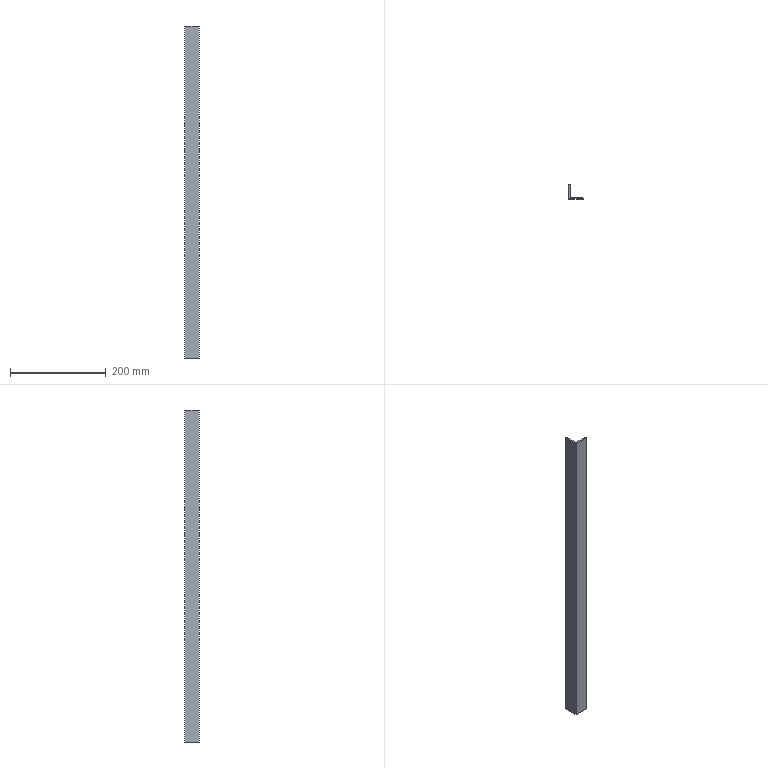Part | SolidWorks | features Extrusion 1 | 1 solid | 11 faces | box 30 x 30 x 692 mm | volume 117738 mm3 | plane 8 | cylinder 3 | commonest cylinder face diameters 4 x3
STEP:
#1=CARTESIAN_POINT('',(0.,30.,0.));
#2=VERTEX_POINT('',#1);
#3=CARTESIAN_POINT('',(0.,0.,0.));
#4=VERTEX_POINT('',#3);
#5=CARTESIAN_POINT('',(0.,0.,0.));
#6=DIRECTION('',(0.,-1.,0.));
#7=VECTOR('',#6,1000.);
#8=LINE('',#5,#7);
#9=EDGE_CURVE('',#2,#4,#8,.T.);
#10=ORIENTED_EDGE('',*,*,#9,.T.);
#11=CARTESIAN_POINT('',(0.,0.,692.));
#12=VERTEX_POINT('',#11);
#13=CARTESIAN_POINT('',(0.,0.,692.));
#14=DIRECTION('',(0.,0.,-1.));
#15=VECTOR('',#14,1000.);
#16=LINE('',#13,#15);
#17=EDGE_CURVE('',#12,#4,#16,.T.);
#18=ORIENTED_EDGE('',*,*,#17,.F.);
#19=CARTESIAN_POINT('',(0.,30.,692.));
#20=VERTEX_POINT('',#19);
#21=CARTESIAN_POINT('',(0.,0.,692.));
#22=DIRECTION('',(0.,-1.,0.));
#23=VECTOR('',#22,1000.);
#24=LINE('',#21,#23);
#25=EDGE_CURVE('',#20,#12,#24,.T.);
#26=ORIENTED_EDGE('',*,*,#25,.F.);
#27=CARTESIAN_POINT('',(0.,30.,692.));
#28=DIRECTION('',(0.,0.,-1.));
#29=VECTOR('',#28,1000.);
#30=LINE('',#27,#29);
#31=EDGE_CURVE('',#20,#2,#30,.T.);
#32=ORIENTED_EDGE('',*,*,#31,.T.);
#33=EDGE_LOOP('',(#10,#18,#26,#32));
#34=FACE_OUTER_BOUND('',#33,.T.);
#35=CARTESIAN_POINT('',(0.,0.,692.));
#36=DIRECTION('',(1.,0.,0.));
#37=DIRECTION('',(0.,0.,-1.));
#38=AXIS2_PLACEMENT_3D('',#35,#36,#37);
#39=PLANE('',#38);
#40=ADVANCED_FACE('',(#34),#39,.F.);
#41=CARTESIAN_POINT('',(30.,0.,0.));
#42=VERTEX_POINT('',#41);
#43=CARTESIAN_POINT('',(0.,0.,0.));
#44=DIRECTION('',(1.,0.,0.));
#45=VECTOR('',#44,1000.);
#46=LINE('',#43,#45);
#47=EDGE_CURVE('',#4,#42,#46,.T.);
#48=ORIENTED_EDGE('',*,*,#47,.T.);
#49=CARTESIAN_POINT('',(30.,0.,692.));
#50=VERTEX_POINT('',#49);
#51=CARTESIAN_POINT('',(30.,0.,692.));
#52=DIRECTION('',(0.,0.,-1.));
#53=VECTOR('',#52,1000.);
#54=LINE('',#51,#53);
#55=EDGE_CURVE('',#50,#42,#54,.T.);
#56=ORIENTED_EDGE('',*,*,#55,.F.);
#57=CARTESIAN_POINT('',(0.,0.,692.));
#58=DIRECTION('',(1.,0.,0.));
#59=VECTOR('',#58,1000.);
#60=LINE('',#57,#59);
#61=EDGE_CURVE('',#12,#50,#60,.T.);
#62=ORIENTED_EDGE('',*,*,#61,.F.);
#63=ORIENTED_EDGE('',*,*,#17,.T.);
#64=EDGE_LOOP('',(#48,#56,#62,#63));
#65=FACE_OUTER_BOUND('',#64,.T.);
#66=CARTESIAN_POINT('',(0.,0.,692.));
#67=DIRECTION('',(0.,1.,0.));
#68=DIRECTION('',(0.,0.,1.));
#69=AXIS2_PLACEMENT_3D('',#66,#67,#68);
#70=PLANE('',#69);
#71=ADVANCED_FACE('',(#65),#70,.F.);
#72=CARTESIAN_POINT('',(30.,1.,0.));
#73=VERTEX_POINT('',#72);
#74=CARTESIAN_POINT('',(30.,1.,0.));
#75=DIRECTION('',(0.,1.,0.));
#76=VECTOR('',#75,1000.);
#77=LINE('',#74,#76);
#78=EDGE_CURVE('',#42,#73,#77,.T.);
#79=ORIENTED_EDGE('',*,*,#78,.T.);
#80=CARTESIAN_POINT('',(30.,1.,692.));
#81=VERTEX_POINT('',#80);
#82=CARTESIAN_POINT('',(30.,1.,692.));
#83=DIRECTION('',(0.,0.,-1.));
#84=VECTOR('',#83,1000.);
#85=LINE('',#82,#84);
#86=EDGE_CURVE('',#81,#73,#85,.T.);
#87=ORIENTED_EDGE('',*,*,#86,.F.);
#88=CARTESIAN_POINT('',(30.,1.,692.));
#89=DIRECTION('',(0.,1.,0.));
#90=VECTOR('',#89,1000.);
#91=LINE('',#88,#90);
#92=EDGE_CURVE('',#50,#81,#91,.T.);
#93=ORIENTED_EDGE('',*,*,#92,.F.);
#94=ORIENTED_EDGE('',*,*,#55,.T.);
#95=EDGE_LOOP('',(#79,#87,#93,#94));
#96=FACE_OUTER_BOUND('',#95,.T.);
#97=CARTESIAN_POINT('',(30.,1.,692.));
#98=DIRECTION('',(-1.,0.,0.));
#99=DIRECTION('',(0.,0.,1.));
#100=AXIS2_PLACEMENT_3D('',#97,#98,#99);
#101=PLANE('',#100);
#102=ADVANCED_FACE('',(#96),#101,.F.);
#103=CARTESIAN_POINT('',(28.,3.,0.));
#104=VERTEX_POINT('',#103);
#105=CARTESIAN_POINT('',(28.,1.,0.));
#106=DIRECTION('',(0.,0.,1.));
#107=DIRECTION('',(1.,0.,0.));
#108=AXIS2_PLACEMENT_3D('',#105,#106,#107);
#109=CIRCLE('',#108,2.);
#110=EDGE_CURVE('',#73,#104,#109,.T.);
#111=ORIENTED_EDGE('',*,*,#110,.T.);
#112=CARTESIAN_POINT('',(28.,3.,692.));
#113=VERTEX_POINT('',#112);
#114=CARTESIAN_POINT('',(28.,3.,692.));
#115=DIRECTION('',(0.,0.,-1.));
#116=VECTOR('',#115,1000.);
#117=LINE('',#114,#116);
#118=EDGE_CURVE('',#113,#104,#117,.T.);
#119=ORIENTED_EDGE('',*,*,#118,.F.);
#120=CARTESIAN_POINT('',(28.,1.,692.));
#121=DIRECTION('',(0.,0.,1.));
#122=DIRECTION('',(1.,0.,0.));
#123=AXIS2_PLACEMENT_3D('',#120,#121,#122);
#124=CIRCLE('',#123,2.);
#125=EDGE_CURVE('',#81,#113,#124,.T.);
#126=ORIENTED_EDGE('',*,*,#125,.F.);
#127=ORIENTED_EDGE('',*,*,#86,.T.);
#128=EDGE_LOOP('',(#111,#119,#126,#127));
#129=FACE_OUTER_BOUND('',#128,.T.);
#130=CARTESIAN_POINT('',(28.,1.,692.));
#131=DIRECTION('',(0.,0.,-1.));
#132=DIRECTION('',(-1.,0.,0.));
#133=AXIS2_PLACEMENT_3D('',#130,#131,#132);
#134=CYLINDRICAL_SURFACE('',#133,2.);
#135=ADVANCED_FACE('',(#129),#134,.T.);
#136=CARTESIAN_POINT('',(5.,3.,0.));
#137=VERTEX_POINT('',#136);
#138=CARTESIAN_POINT('',(5.,3.,0.));
#139=DIRECTION('',(-1.,0.,0.));
#140=VECTOR('',#139,1000.);
#141=LINE('',#138,#140);
#142=EDGE_CURVE('',#104,#137,#141,.T.);
#143=ORIENTED_EDGE('',*,*,#142,.T.);
#144=CARTESIAN_POINT('',(5.,3.,692.));
#145=VERTEX_POINT('',#144);
#146=CARTESIAN_POINT('',(5.,3.,692.));
#147=DIRECTION('',(0.,0.,-1.));
#148=VECTOR('',#147,1000.);
#149=LINE('',#146,#148);
#150=EDGE_CURVE('',#145,#137,#149,.T.);
#151=ORIENTED_EDGE('',*,*,#150,.F.);
#152=CARTESIAN_POINT('',(5.,3.,692.));
#153=DIRECTION('',(-1.,0.,0.));
#154=VECTOR('',#153,1000.);
#155=LINE('',#152,#154);
#156=EDGE_CURVE('',#113,#145,#155,.T.);
#157=ORIENTED_EDGE('',*,*,#156,.F.);
#158=ORIENTED_EDGE('',*,*,#118,.T.);
#159=EDGE_LOOP('',(#143,#151,#157,#158));
#160=FACE_OUTER_BOUND('',#159,.T.);
#161=CARTESIAN_POINT('',(5.,3.,692.));
#162=DIRECTION('',(0.,-1.,0.));
#163=DIRECTION('',(0.,0.,-1.));
#164=AXIS2_PLACEMENT_3D('',#161,#162,#163);
#165=PLANE('',#164);
#166=ADVANCED_FACE('',(#160),#165,.F.);
#167=CARTESIAN_POINT('',(3.,5.,0.));
#168=VERTEX_POINT('',#167);
#169=CARTESIAN_POINT('',(5.,5.,0.));
#170=DIRECTION('',(0.,0.,-1.));
#171=DIRECTION('',(-1.,0.,0.));
#172=AXIS2_PLACEMENT_3D('',#169,#170,#171);
#173=CIRCLE('',#172,2.);
#174=EDGE_CURVE('',#137,#168,#173,.T.);
#175=ORIENTED_EDGE('',*,*,#174,.T.);
#176=CARTESIAN_POINT('',(3.,5.,692.));
#177=VERTEX_POINT('',#176);
#178=CARTESIAN_POINT('',(3.,5.,692.));
#179=DIRECTION('',(0.,0.,-1.));
#180=VECTOR('',#179,1000.);
#181=LINE('',#178,#180);
#182=EDGE_CURVE('',#177,#168,#181,.T.);
#183=ORIENTED_EDGE('',*,*,#182,.F.);
#184=CARTESIAN_POINT('',(5.,5.,692.));
#185=DIRECTION('',(0.,0.,-1.));
#186=DIRECTION('',(-1.,0.,0.));
#187=AXIS2_PLACEMENT_3D('',#184,#185,#186);
#188=CIRCLE('',#187,2.);
#189=EDGE_CURVE('',#145,#177,#188,.T.);
#190=ORIENTED_EDGE('',*,*,#189,.F.);
#191=ORIENTED_EDGE('',*,*,#150,.T.);
#192=EDGE_LOOP('',(#175,#183,#190,#191));
#193=FACE_OUTER_BOUND('',#192,.T.);
#194=CARTESIAN_POINT('',(5.,5.,692.));
#195=DIRECTION('',(0.,0.,-1.));
#196=DIRECTION('',(-1.,0.,0.));
#197=AXIS2_PLACEMENT_3D('',#194,#195,#196);
#198=CYLINDRICAL_SURFACE('',#197,2.);
#199=ADVANCED_FACE('',(#193),#198,.F.);
#200=CARTESIAN_POINT('',(3.,28.,0.));
#201=VERTEX_POINT('',#200);
#202=CARTESIAN_POINT('',(3.,5.,0.));
#203=DIRECTION('',(0.,1.,0.));
#204=VECTOR('',#203,1000.);
#205=LINE('',#202,#204);
#206=EDGE_CURVE('',#168,#201,#205,.T.);
#207=ORIENTED_EDGE('',*,*,#206,.T.);
#208=CARTESIAN_POINT('',(3.,28.,692.));
#209=VERTEX_POINT('',#208);
#210=CARTESIAN_POINT('',(3.,28.,692.));
#211=DIRECTION('',(0.,0.,-1.));
#212=VECTOR('',#211,1000.);
#213=LINE('',#210,#212);
#214=EDGE_CURVE('',#209,#201,#213,.T.);
#215=ORIENTED_EDGE('',*,*,#214,.F.);
#216=CARTESIAN_POINT('',(3.,5.,692.));
#217=DIRECTION('',(0.,1.,0.));
#218=VECTOR('',#217,1000.);
#219=LINE('',#216,#218);
#220=EDGE_CURVE('',#177,#209,#219,.T.);
#221=ORIENTED_EDGE('',*,*,#220,.F.);
#222=ORIENTED_EDGE('',*,*,#182,.T.);
#223=EDGE_LOOP('',(#207,#215,#221,#222));
#224=FACE_OUTER_BOUND('',#223,.T.);
#225=CARTESIAN_POINT('',(3.,5.,692.));
#226=DIRECTION('',(-1.,0.,0.));
#227=DIRECTION('',(0.,0.,1.));
#228=AXIS2_PLACEMENT_3D('',#225,#226,#227);
#229=PLANE('',#228);
#230=ADVANCED_FACE('',(#224),#229,.F.);
#231=CARTESIAN_POINT('',(1.,30.,0.));
#232=VERTEX_POINT('',#231);
#233=CARTESIAN_POINT('',(1.,28.,0.));
#234=DIRECTION('',(0.,0.,1.));
#235=DIRECTION('',(1.,0.,0.));
#236=AXIS2_PLACEMENT_3D('',#233,#234,#235);
#237=CIRCLE('',#236,2.);
#238=EDGE_CURVE('',#201,#232,#237,.T.);
#239=ORIENTED_EDGE('',*,*,#238,.T.);
#240=CARTESIAN_POINT('',(1.,30.,692.));
#241=VERTEX_POINT('',#240);
#242=CARTESIAN_POINT('',(1.,30.,692.));
#243=DIRECTION('',(0.,0.,-1.));
#244=VECTOR('',#243,1000.);
#245=LINE('',#242,#244);
#246=EDGE_CURVE('',#241,#232,#245,.T.);
#247=ORIENTED_EDGE('',*,*,#246,.F.);
#248=CARTESIAN_POINT('',(1.,28.,692.));
#249=DIRECTION('',(0.,0.,1.));
#250=DIRECTION('',(1.,0.,0.));
#251=AXIS2_PLACEMENT_3D('',#248,#249,#250);
#252=CIRCLE('',#251,2.);
#253=EDGE_CURVE('',#209,#241,#252,.T.);
#254=ORIENTED_EDGE('',*,*,#253,.F.);
#255=ORIENTED_EDGE('',*,*,#214,.T.);
#256=EDGE_LOOP('',(#239,#247,#254,#255));
#257=FACE_OUTER_BOUND('',#256,.T.);
#258=CARTESIAN_POINT('',(1.,28.,692.));
#259=DIRECTION('',(0.,0.,-1.));
#260=DIRECTION('',(-1.,0.,0.));
#261=AXIS2_PLACEMENT_3D('',#258,#259,#260);
#262=CYLINDRICAL_SURFACE('',#261,2.);
#263=ADVANCED_FACE('',(#257),#262,.T.);
#264=CARTESIAN_POINT('',(0.,30.,0.));
#265=DIRECTION('',(-1.,0.,0.));
#266=VECTOR('',#265,1000.);
#267=LINE('',#264,#266);
#268=EDGE_CURVE('',#232,#2,#267,.T.);
#269=ORIENTED_EDGE('',*,*,#268,.T.);
#270=ORIENTED_EDGE('',*,*,#31,.F.);
#271=CARTESIAN_POINT('',(0.,30.,692.));
#272=DIRECTION('',(-1.,0.,0.));
#273=VECTOR('',#272,1000.);
#274=LINE('',#271,#273);
#275=EDGE_CURVE('',#241,#20,#274,.T.);
#276=ORIENTED_EDGE('',*,*,#275,.F.);
#277=ORIENTED_EDGE('',*,*,#246,.T.);
#278=EDGE_LOOP('',(#269,#270,#276,#277));
#279=FACE_OUTER_BOUND('',#278,.T.);
#280=CARTESIAN_POINT('',(0.,30.,692.));
#281=DIRECTION('',(0.,-1.,0.));
#282=DIRECTION('',(0.,0.,-1.));
#283=AXIS2_PLACEMENT_3D('',#280,#281,#282);
#284=PLANE('',#283);
#285=ADVANCED_FACE('',(#279),#284,.F.);
#286=ORIENTED_EDGE('',*,*,#25,.T.);
#287=ORIENTED_EDGE('',*,*,#61,.T.);
#288=ORIENTED_EDGE('',*,*,#92,.T.);
#289=ORIENTED_EDGE('',*,*,#125,.T.);
#290=ORIENTED_EDGE('',*,*,#156,.T.);
#291=ORIENTED_EDGE('',*,*,#189,.T.);
#292=ORIENTED_EDGE('',*,*,#220,.T.);
#293=ORIENTED_EDGE('',*,*,#253,.T.);
#294=ORIENTED_EDGE('',*,*,#275,.T.);
#295=EDGE_LOOP('',(#286,#287,#288,#289,#290,#291,#292,#293,#294));
#296=FACE_OUTER_BOUND('',#295,.T.);
#297=CARTESIAN_POINT('',(1.,28.,692.));
#298=DIRECTION('',(0.,0.,1.));
#299=DIRECTION('',(1.,0.,0.));
#300=AXIS2_PLACEMENT_3D('',#297,#298,#299);
#301=PLANE('',#300);
#302=ADVANCED_FACE('',(#296),#301,.T.);
#303=ORIENTED_EDGE('',*,*,#9,.F.);
#304=ORIENTED_EDGE('',*,*,#268,.F.);
#305=ORIENTED_EDGE('',*,*,#238,.F.);
#306=ORIENTED_EDGE('',*,*,#206,.F.);
#307=ORIENTED_EDGE('',*,*,#174,.F.);
#308=ORIENTED_EDGE('',*,*,#142,.F.);
#309=ORIENTED_EDGE('',*,*,#110,.F.);
#310=ORIENTED_EDGE('',*,*,#78,.F.);
#311=ORIENTED_EDGE('',*,*,#47,.F.);
#312=EDGE_LOOP('',(#303,#304,#305,#306,#307,#308,#309,#310,#311));
#313=FACE_OUTER_BOUND('',#312,.T.);
#314=CARTESIAN_POINT('',(1.,28.,0.));
#315=DIRECTION('',(0.,0.,1.));
#316=DIRECTION('',(1.,0.,0.));
#317=AXIS2_PLACEMENT_3D('',#314,#315,#316);
#318=PLANE('',#317);
#319=ADVANCED_FACE('',(#313),#318,.F.);
#320=CLOSED_SHELL('',(#40,#71,#102,#135,#166,#199,#230,#263,#285,#302,#319));
#321=MANIFOLD_SOLID_BREP('',#320);
#322=CARTESIAN_POINT('',(0.,0.,0.));
#323=DIRECTION('',(0.,0.,1.));
#324=DIRECTION('',(1.,0.,0.));
#325=AXIS2_PLACEMENT_3D('',#322,#323,#324);
#326=(LENGTH_UNIT()NAMED_UNIT(*)SI_UNIT(.MILLI.,.METRE.));
#327=UNCERTAINTY_MEASURE_WITH_UNIT(LENGTH_MEASURE(0.00001),#326,'','');
#328=(NAMED_UNIT(*)PLANE_ANGLE_UNIT()SI_UNIT($,.RADIAN.));
#329=(NAMED_UNIT(*)SI_UNIT($,.STERADIAN.)SOLID_ANGLE_UNIT());
#330=(GEOMETRIC_REPRESENTATION_CONTEXT(3)GLOBAL_UNCERTAINTY_ASSIGNED_CONTEXT((#327))GLOBAL_UNIT_ASSIGNED_CONTEXT((#326,#328,#329))REPRESENTATION_CONTEXT('',''));
#331=ADVANCED_BREP_SHAPE_REPRESENTATION('',(#321,#325),#330);